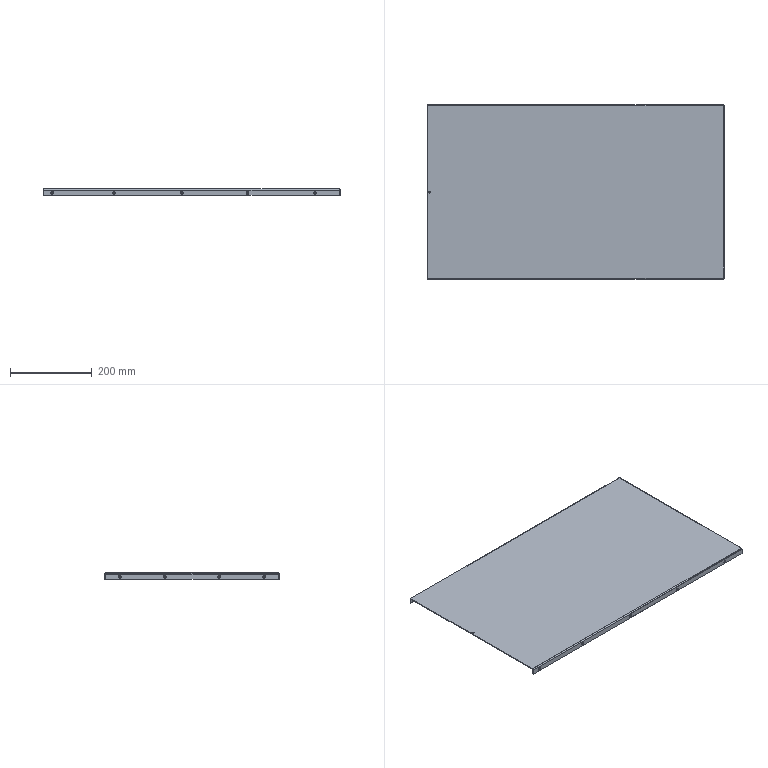Part | NX | features BREP 1 | 1 solid | 86 faces | box 724.237 x 425.821 x 15 mm | volume 661919 mm3 | cylinder 34 | cone 28 | plane 20 | spline 4 | commonest cylinder face diameters 3.4 x27 1.473 x3 5.473 x3 3 x1